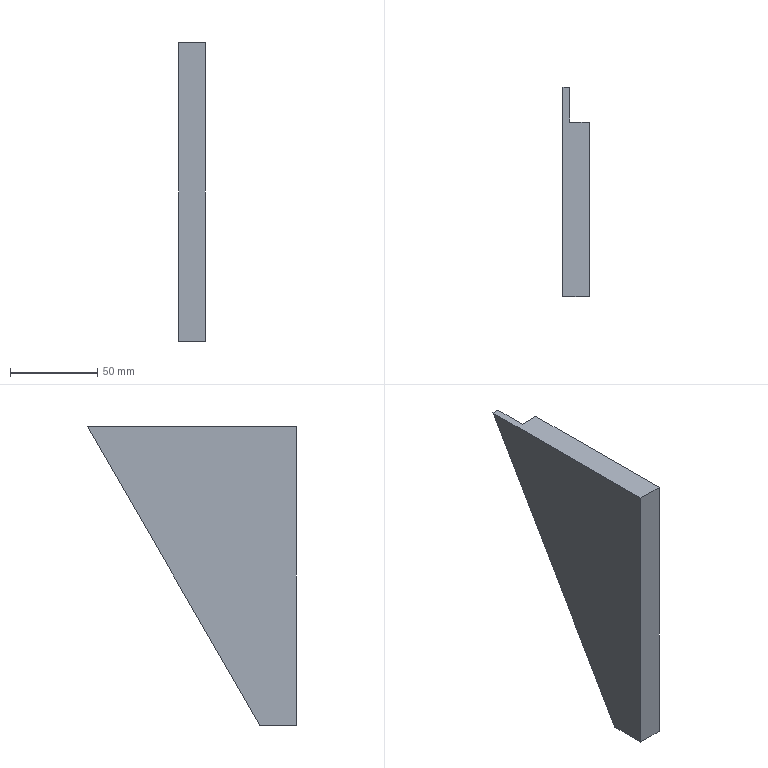Part | STEP file | 02-21 Push plate | 1 solid | 16 faces | box 15 x 120 x 171.5 mm | volume 143256 mm3 | plane 8 | cylinder 4 | cone 4 | commonest cylinder face diameters 4.2 x4
STEP:
#1=CARTESIAN_POINT('',(0.,0.,0.));
#2=DIRECTION('',(0.,0.,1.));
#3=DIRECTION('',(1.,0.,0.));
#4=AXIS2_PLACEMENT_3D('',#1,#2,#3);
#5=CARTESIAN_POINT('',(2.6,22.5,-67.6));
#6=VERTEX_POINT('',#5);
#7=CARTESIAN_POINT('',(15.,22.5,-67.6));
#8=VERTEX_POINT('',#7);
#9=CARTESIAN_POINT('',(2.6,22.5,-67.6));
#10=DIRECTION('',(1.,0.,0.));
#11=VECTOR('',#10,1.);
#12=LINE('',#9,#11);
#13=CARTESIAN_POINT('',(2.6,22.5,-65.5));
#14=DIRECTION('',(1.,0.,0.));
#15=DIRECTION('',(0.,0.,-1.));
#16=AXIS2_PLACEMENT_3D('',#13,#14,#15);
#17=CYLINDRICAL_SURFACE('',#16,2.1);
#18=CARTESIAN_POINT('',(6.283,0.));
#19=DIRECTION('',(0.,1.));
#20=VECTOR('',#19,1.);
#21=LINE('',#18,#20);
#22=(GEOMETRIC_REPRESENTATION_CONTEXT(2)PARAMETRIC_REPRESENTATION_CONTEXT()REPRESENTATION_CONTEXT('',''));
#23=DEFINITIONAL_REPRESENTATION('',(#21),#22);
#24=PCURVE('',#17,#23);
#25=CARTESIAN_POINT('',(2.6,22.5,-65.5));
#26=DIRECTION('',(1.,0.,0.));
#27=DIRECTION('',(0.,0.,-1.));
#28=AXIS2_PLACEMENT_3D('',#25,#26,#27);
#29=CYLINDRICAL_SURFACE('',#28,2.1);
#30=CARTESIAN_POINT('',(0.,0.));
#31=DIRECTION('',(0.,1.));
#32=VECTOR('',#31,1.);
#33=LINE('',#30,#32);
#34=(GEOMETRIC_REPRESENTATION_CONTEXT(2)PARAMETRIC_REPRESENTATION_CONTEXT()REPRESENTATION_CONTEXT('',''));
#35=DEFINITIONAL_REPRESENTATION('',(#33),#34);
#36=PCURVE('',#29,#35);
#37=SURFACE_CURVE('',#12,(#24,#36),.PCURVE_S1.);
#38=EDGE_CURVE('',#6,#8,#37,.T.);
#39=ORIENTED_EDGE('',*,*,#38,.T.);
#40=CARTESIAN_POINT('',(15.,22.5,-63.4));
#41=VERTEX_POINT('',#40);
#42=CARTESIAN_POINT('',(15.,22.5,-65.5));
#43=DIRECTION('',(1.,0.,0.));
#44=DIRECTION('',(0.,0.,-1.));
#45=AXIS2_PLACEMENT_3D('',#42,#43,#44);
#46=CIRCLE('',#45,2.1);
#47=CARTESIAN_POINT('',(0.,12.4));
#48=DIRECTION('',(1.,0.));
#49=VECTOR('',#48,1.);
#50=LINE('',#47,#49);
#51=(GEOMETRIC_REPRESENTATION_CONTEXT(2)PARAMETRIC_REPRESENTATION_CONTEXT()REPRESENTATION_CONTEXT('',''));
#52=DEFINITIONAL_REPRESENTATION('',(#50),#51);
#53=PCURVE('',#17,#52);
#54=CARTESIAN_POINT('',(15.,0.,-171.5));
#55=DIRECTION('',(-1.,0.,0.));
#56=DIRECTION('',(0.,0.,1.));
#57=AXIS2_PLACEMENT_3D('',#54,#55,#56);
#58=PLANE('',#57);
#59=CARTESIAN_POINT('',(103.9,22.5));
#60=CARTESIAN_POINT('',(103.9,26.137));
#61=CARTESIAN_POINT('',(107.05,24.319));
#62=CARTESIAN_POINT('',(110.2,22.5));
#63=CARTESIAN_POINT('',(107.05,20.681));
#64=CARTESIAN_POINT('',(103.9,18.863));
#65=CARTESIAN_POINT('',(103.9,22.5));
#66=(BOUNDED_CURVE()B_SPLINE_CURVE(2,(#59,#60,#61,#62,#63,#64,#65),.UNSPECIFIED.,.T.,.F.)B_SPLINE_CURVE_WITH_KNOTS((1,2,2,2,2,1),(-2.094,0.,2.094,4.189,6.283,8.378),.UNSPECIFIED.)CURVE()GEOMETRIC_REPRESENTATION_ITEM()RATIONAL_B_SPLINE_CURVE((1.,0.5,1.,0.5,1.,0.5,1.))REPRESENTATION_ITEM(''));
#67=(GEOMETRIC_REPRESENTATION_CONTEXT(2)PARAMETRIC_REPRESENTATION_CONTEXT()REPRESENTATION_CONTEXT('',''));
#68=DEFINITIONAL_REPRESENTATION('',(#66),#67);
#69=PCURVE('',#58,#68);
#70=SURFACE_CURVE('',#46,(#53,#69),.PCURVE_S1.);
#71=EDGE_CURVE('',#41,#8,#70,.T.);
#72=ORIENTED_EDGE('',*,*,#71,.F.);
#73=CARTESIAN_POINT('',(2.6,22.5,-63.4));
#74=VERTEX_POINT('',#73);
#75=CARTESIAN_POINT('',(2.6,22.5,-63.4));
#76=DIRECTION('',(1.,0.,0.));
#77=VECTOR('',#76,1.);
#78=LINE('',#75,#77);
#79=CARTESIAN_POINT('',(3.142,0.));
#80=DIRECTION('',(0.,1.));
#81=VECTOR('',#80,1.);
#82=LINE('',#79,#81);
#83=(GEOMETRIC_REPRESENTATION_CONTEXT(2)PARAMETRIC_REPRESENTATION_CONTEXT()REPRESENTATION_CONTEXT('',''));
#84=DEFINITIONAL_REPRESENTATION('',(#82),#83);
#85=PCURVE('',#17,#84);
#86=CARTESIAN_POINT('',(3.142,0.));
#87=DIRECTION('',(0.,1.));
#88=VECTOR('',#87,1.);
#89=LINE('',#86,#88);
#90=(GEOMETRIC_REPRESENTATION_CONTEXT(2)PARAMETRIC_REPRESENTATION_CONTEXT()REPRESENTATION_CONTEXT('',''));
#91=DEFINITIONAL_REPRESENTATION('',(#89),#90);
#92=PCURVE('',#29,#91);
#93=SURFACE_CURVE('',#78,(#85,#92),.PCURVE_S1.);
#94=EDGE_CURVE('',#74,#41,#93,.T.);
#95=ORIENTED_EDGE('',*,*,#94,.F.);
#96=CARTESIAN_POINT('',(2.6,22.5,-65.5));
#97=DIRECTION('',(-1.,0.,0.));
#98=DIRECTION('',(0.,0.,-1.));
#99=AXIS2_PLACEMENT_3D('',#96,#97,#98);
#100=CIRCLE('',#99,2.1);
#101=CARTESIAN_POINT('',(6.283,0.));
#102=DIRECTION('',(-1.,0.));
#103=VECTOR('',#102,1.);
#104=LINE('',#101,#103);
#105=(GEOMETRIC_REPRESENTATION_CONTEXT(2)PARAMETRIC_REPRESENTATION_CONTEXT()REPRESENTATION_CONTEXT('',''));
#106=DEFINITIONAL_REPRESENTATION('',(#104),#105);
#107=PCURVE('',#17,#106);
#108=CARTESIAN_POINT('',(1001.338,22.5,-65.5));
#109=DIRECTION('',(1.,0.,0.));
#110=DIRECTION('',(0.,0.,-1.));
#111=AXIS2_PLACEMENT_3D('',#108,#109,#110);
#112=CONICAL_SURFACE('',#111,1664.279,1.03);
#113=CARTESIAN_POINT('',(6.283,-998.738));
#114=DIRECTION('',(-1.,0.));
#115=VECTOR('',#114,1.);
#116=LINE('',#113,#115);
#117=(GEOMETRIC_REPRESENTATION_CONTEXT(2)PARAMETRIC_REPRESENTATION_CONTEXT()REPRESENTATION_CONTEXT('',''));
#118=DEFINITIONAL_REPRESENTATION('',(#116),#117);
#119=PCURVE('',#112,#118);
#120=SURFACE_CURVE('',#100,(#107,#119),.PCURVE_S1.);
#121=EDGE_CURVE('',#6,#74,#120,.T.);
#122=ORIENTED_EDGE('',*,*,#121,.F.);
#123=EDGE_LOOP('',(#39,#72,#95,#122));
#124=FACE_BOUND('',#123,.F.);
#125=ADVANCED_FACE('',(#124),#17,.F.);
#126=ORIENTED_EDGE('',*,*,#121,.T.);
#127=CARTESIAN_POINT('',(1.338,22.5,-65.5));
#128=VERTEX_POINT('',#127);
#129=CARTESIAN_POINT('',(1.338,22.5,-65.5));
#130=DIRECTION('',(0.515,0.,0.8572));
#131=VECTOR('',#130,1.);
#132=LINE('',#129,#131);
#133=CARTESIAN_POINT('',(3.142,-1000.));
#134=CARTESIAN_POINT('',(3.142,-999.981));
#135=CARTESIAN_POINT('',(3.142,-999.943));
#136=CARTESIAN_POINT('',(3.142,-999.885));
#137=CARTESIAN_POINT('',(3.142,-999.828));
#138=CARTESIAN_POINT('',(3.142,-999.771));
#139=CARTESIAN_POINT('',(3.142,-999.713));
#140=CARTESIAN_POINT('',(3.142,-999.656));
#141=CARTESIAN_POINT('',(3.142,-999.599));
#142=CARTESIAN_POINT('',(3.142,-999.541));
#143=CARTESIAN_POINT('',(3.142,-999.484));
#144=CARTESIAN_POINT('',(3.142,-999.426));
#145=CARTESIAN_POINT('',(3.142,-999.369));
#146=CARTESIAN_POINT('',(3.142,-999.312));
#147=CARTESIAN_POINT('',(3.142,-999.254));
#148=CARTESIAN_POINT('',(3.142,-999.197));
#149=CARTESIAN_POINT('',(3.142,-999.14));
#150=CARTESIAN_POINT('',(3.142,-999.082));
#151=CARTESIAN_POINT('',(3.142,-999.025));
#152=CARTESIAN_POINT('',(3.142,-998.968));
#153=CARTESIAN_POINT('',(3.142,-998.91));
#154=CARTESIAN_POINT('',(3.142,-998.853));
#155=CARTESIAN_POINT('',(3.142,-998.796));
#156=CARTESIAN_POINT('',(3.142,-998.757));
#157=CARTESIAN_POINT('',(3.142,-998.738));
#158=B_SPLINE_CURVE_WITH_KNOTS('',3,(#133,#134,#135,#136,#137,#138,#139,#140,#141,#142,#143,#144,#145,#146,#147,#148,#149,#150,#151,#152,#153,#154,#155,#156,#157),.UNSPECIFIED.,.F.,.F.,(4,1,1,1,1,1,1,1,1,1,1,1,1,1,1,1,1,1,1,1,1,1,4),(0.,0.1114,0.2227,0.3341,0.4454,0.5568,0.6682,0.7795,0.8909,1.002,1.114,1.225,1.336,1.448,1.559,1.67,1.782,1.893,2.004,2.116,2.227,2.339,2.45),.QUASI_UNIFORM_KNOTS.);
#159=(GEOMETRIC_REPRESENTATION_CONTEXT(2)PARAMETRIC_REPRESENTATION_CONTEXT()REPRESENTATION_CONTEXT('',''));
#160=DEFINITIONAL_REPRESENTATION('',(#158),#159);
#161=PCURVE('',#112,#160);
#162=CARTESIAN_POINT('',(1001.338,22.5,-65.5));
#163=DIRECTION('',(1.,0.,0.));
#164=DIRECTION('',(0.,0.,-1.));
#165=AXIS2_PLACEMENT_3D('',#162,#163,#164);
#166=CONICAL_SURFACE('',#165,1664.279,1.03);
#167=CARTESIAN_POINT('',(3.142,-1000.));
#168=CARTESIAN_POINT('',(3.142,-999.981));
#169=CARTESIAN_POINT('',(3.142,-999.943));
#170=CARTESIAN_POINT('',(3.142,-999.885));
#171=CARTESIAN_POINT('',(3.142,-999.828));
#172=CARTESIAN_POINT('',(3.142,-999.771));
#173=CARTESIAN_POINT('',(3.142,-999.713));
#174=CARTESIAN_POINT('',(3.142,-999.656));
#175=CARTESIAN_POINT('',(3.142,-999.599));
#176=CARTESIAN_POINT('',(3.142,-999.541));
#177=CARTESIAN_POINT('',(3.142,-999.484));
#178=CARTESIAN_POINT('',(3.142,-999.426));
#179=CARTESIAN_POINT('',(3.142,-999.369));
#180=CARTESIAN_POINT('',(3.142,-999.312));
#181=CARTESIAN_POINT('',(3.142,-999.254));
#182=CARTESIAN_POINT('',(3.142,-999.197));
#183=CARTESIAN_POINT('',(3.142,-999.14));
#184=CARTESIAN_POINT('',(3.142,-999.082));
#185=CARTESIAN_POINT('',(3.142,-999.025));
#186=CARTESIAN_POINT('',(3.142,-998.968));
#187=CARTESIAN_POINT('',(3.142,-998.91));
#188=CARTESIAN_POINT('',(3.142,-998.853));
#189=CARTESIAN_POINT('',(3.142,-998.796));
#190=CARTESIAN_POINT('',(3.142,-998.757));
#191=CARTESIAN_POINT('',(3.142,-998.738));
#192=B_SPLINE_CURVE_WITH_KNOTS('',3,(#167,#168,#169,#170,#171,#172,#173,#174,#175,#176,#177,#178,#179,#180,#181,#182,#183,#184,#185,#186,#187,#188,#189,#190,#191),.UNSPECIFIED.,.F.,.F.,(4,1,1,1,1,1,1,1,1,1,1,1,1,1,1,1,1,1,1,1,1,1,4),(0.,0.1114,0.2227,0.3341,0.4454,0.5568,0.6682,0.7795,0.8909,1.002,1.114,1.225,1.336,1.448,1.559,1.67,1.782,1.893,2.004,2.116,2.227,2.339,2.45),.QUASI_UNIFORM_KNOTS.);
#193=(GEOMETRIC_REPRESENTATION_CONTEXT(2)PARAMETRIC_REPRESENTATION_CONTEXT()REPRESENTATION_CONTEXT('',''));
#194=DEFINITIONAL_REPRESENTATION('',(#192),#193);
#195=PCURVE('',#166,#194);
#196=SURFACE_CURVE('',#132,(#161,#195),.PCURVE_S1.);
#197=EDGE_CURVE('',#128,#74,#196,.T.);
#198=ORIENTED_EDGE('',*,*,#197,.F.);
#199=CARTESIAN_POINT('',(1.338,22.5,-65.5));
#200=DIRECTION('',(0.515,0.,-0.8572));
#201=VECTOR('',#200,1.);
#202=LINE('',#199,#201);
#203=CARTESIAN_POINT('',(6.283,-1000.));
#204=DIRECTION('',(0.,1.));
#205=VECTOR('',#204,1.);
#206=LINE('',#203,#205);
#207=(GEOMETRIC_REPRESENTATION_CONTEXT(2)PARAMETRIC_REPRESENTATION_CONTEXT()REPRESENTATION_CONTEXT('',''));
#208=DEFINITIONAL_REPRESENTATION('',(#206),#207);
#209=PCURVE('',#112,#208);
#210=CARTESIAN_POINT('',(0.,-1000.));
#211=DIRECTION('',(0.,1.));
#212=VECTOR('',#211,1.);
#213=LINE('',#210,#212);
#214=(GEOMETRIC_REPRESENTATION_CONTEXT(2)PARAMETRIC_REPRESENTATION_CONTEXT()REPRESENTATION_CONTEXT('',''));
#215=DEFINITIONAL_REPRESENTATION('',(#213),#214);
#216=PCURVE('',#166,#215);
#217=SURFACE_CURVE('',#202,(#209,#216),.PCURVE_S1.);
#218=EDGE_CURVE('',#128,#6,#217,.T.);
#219=ORIENTED_EDGE('',*,*,#218,.T.);
#220=EDGE_LOOP('',(#126,#198,#219));
#221=FACE_BOUND('',#220,.F.);
#222=ADVANCED_FACE('',(#221),#112,.F.);
#223=CARTESIAN_POINT('',(2.6,22.5,-97.6));
#224=VERTEX_POINT('',#223);
#225=CARTESIAN_POINT('',(15.,22.5,-97.6));
#226=VERTEX_POINT('',#225);
#227=CARTESIAN_POINT('',(2.6,22.5,-97.6));
#228=DIRECTION('',(1.,0.,0.));
#229=VECTOR('',#228,1.);
#230=LINE('',#227,#229);
#231=CARTESIAN_POINT('',(2.6,22.5,-95.5));
#232=DIRECTION('',(1.,0.,0.));
#233=DIRECTION('',(0.,0.,-1.));
#234=AXIS2_PLACEMENT_3D('',#231,#232,#233);
#235=CYLINDRICAL_SURFACE('',#234,2.1);
#236=CARTESIAN_POINT('',(6.283,0.));
#237=DIRECTION('',(0.,1.));
#238=VECTOR('',#237,1.);
#239=LINE('',#236,#238);
#240=(GEOMETRIC_REPRESENTATION_CONTEXT(2)PARAMETRIC_REPRESENTATION_CONTEXT()REPRESENTATION_CONTEXT('',''));
#241=DEFINITIONAL_REPRESENTATION('',(#239),#240);
#242=PCURVE('',#235,#241);
#243=CARTESIAN_POINT('',(2.6,22.5,-95.5));
#244=DIRECTION('',(1.,0.,0.));
#245=DIRECTION('',(0.,0.,-1.));
#246=AXIS2_PLACEMENT_3D('',#243,#244,#245);
#247=CYLINDRICAL_SURFACE('',#246,2.1);
#248=CARTESIAN_POINT('',(0.,0.));
#249=DIRECTION('',(0.,1.));
#250=VECTOR('',#249,1.);
#251=LINE('',#248,#250);
#252=(GEOMETRIC_REPRESENTATION_CONTEXT(2)PARAMETRIC_REPRESENTATION_CONTEXT()REPRESENTATION_CONTEXT('',''));
#253=DEFINITIONAL_REPRESENTATION('',(#251),#252);
#254=PCURVE('',#247,#253);
#255=SURFACE_CURVE('',#230,(#242,#254),.PCURVE_S1.);
#256=EDGE_CURVE('',#224,#226,#255,.T.);
#257=ORIENTED_EDGE('',*,*,#256,.T.);
#258=CARTESIAN_POINT('',(15.,22.5,-93.4));
#259=VERTEX_POINT('',#258);
#260=CARTESIAN_POINT('',(15.,22.5,-95.5));
#261=DIRECTION('',(1.,0.,0.));
#262=DIRECTION('',(0.,0.,-1.));
#263=AXIS2_PLACEMENT_3D('',#260,#261,#262);
#264=CIRCLE('',#263,2.1);
#265=CARTESIAN_POINT('',(0.,12.4));
#266=DIRECTION('',(1.,0.));
#267=VECTOR('',#266,1.);
#268=LINE('',#265,#267);
#269=(GEOMETRIC_REPRESENTATION_CONTEXT(2)PARAMETRIC_REPRESENTATION_CONTEXT()REPRESENTATION_CONTEXT('',''));
#270=DEFINITIONAL_REPRESENTATION('',(#268),#269);
#271=PCURVE('',#235,#270);
#272=CARTESIAN_POINT('',(73.9,22.5));
#273=CARTESIAN_POINT('',(73.9,26.137));
#274=CARTESIAN_POINT('',(77.05,24.319));
#275=CARTESIAN_POINT('',(80.2,22.5));
#276=CARTESIAN_POINT('',(77.05,20.681));
#277=CARTESIAN_POINT('',(73.9,18.863));
#278=CARTESIAN_POINT('',(73.9,22.5));
#279=(BOUNDED_CURVE()B_SPLINE_CURVE(2,(#272,#273,#274,#275,#276,#277,#278),.UNSPECIFIED.,.T.,.F.)B_SPLINE_CURVE_WITH_KNOTS((1,2,2,2,2,1),(-2.094,0.,2.094,4.189,6.283,8.378),.UNSPECIFIED.)CURVE()GEOMETRIC_REPRESENTATION_ITEM()RATIONAL_B_SPLINE_CURVE((1.,0.5,1.,0.5,1.,0.5,1.))REPRESENTATION_ITEM(''));
#280=(GEOMETRIC_REPRESENTATION_CONTEXT(2)PARAMETRIC_REPRESENTATION_CONTEXT()REPRESENTATION_CONTEXT('',''));
#281=DEFINITIONAL_REPRESENTATION('',(#279),#280);
#282=PCURVE('',#58,#281);
#283=SURFACE_CURVE('',#264,(#271,#282),.PCURVE_S1.);
#284=EDGE_CURVE('',#259,#226,#283,.T.);
#285=ORIENTED_EDGE('',*,*,#284,.F.);
#286=CARTESIAN_POINT('',(2.6,22.5,-93.4));
#287=VERTEX_POINT('',#286);
#288=CARTESIAN_POINT('',(2.6,22.5,-93.4));
#289=DIRECTION('',(1.,0.,0.));
#290=VECTOR('',#289,1.);
#291=LINE('',#288,#290);
#292=CARTESIAN_POINT('',(3.142,0.));
#293=DIRECTION('',(0.,1.));
#294=VECTOR('',#293,1.);
#295=LINE('',#292,#294);
#296=(GEOMETRIC_REPRESENTATION_CONTEXT(2)PARAMETRIC_REPRESENTATION_CONTEXT()REPRESENTATION_CONTEXT('',''));
#297=DEFINITIONAL_REPRESENTATION('',(#295),#296);
#298=PCURVE('',#235,#297);
#299=CARTESIAN_POINT('',(3.142,0.));
#300=DIRECTION('',(0.,1.));
#301=VECTOR('',#300,1.);
#302=LINE('',#299,#301);
#303=(GEOMETRIC_REPRESENTATION_CONTEXT(2)PARAMETRIC_REPRESENTATION_CONTEXT()REPRESENTATION_CONTEXT('',''));
#304=DEFINITIONAL_REPRESENTATION('',(#302),#303);
#305=PCURVE('',#247,#304);
#306=SURFACE_CURVE('',#291,(#298,#305),.PCURVE_S1.);
#307=EDGE_CURVE('',#287,#259,#306,.T.);
#308=ORIENTED_EDGE('',*,*,#307,.F.);
#309=CARTESIAN_POINT('',(2.6,22.5,-95.5));
#310=DIRECTION('',(-1.,0.,0.));
#311=DIRECTION('',(0.,0.,-1.));
#312=AXIS2_PLACEMENT_3D('',#309,#310,#311);
#313=CIRCLE('',#312,2.1);
#314=CARTESIAN_POINT('',(6.283,0.));
#315=DIRECTION('',(-1.,0.));
#316=VECTOR('',#315,1.);
#317=LINE('',#314,#316);
#318=(GEOMETRIC_REPRESENTATION_CONTEXT(2)PARAMETRIC_REPRESENTATION_CONTEXT()REPRESENTATION_CONTEXT('',''));
#319=DEFINITIONAL_REPRESENTATION('',(#317),#318);
#320=PCURVE('',#235,#319);
#321=CARTESIAN_POINT('',(1001.338,22.5,-95.5));
#322=DIRECTION('',(1.,0.,0.));
#323=DIRECTION('',(0.,0.,-1.));
#324=AXIS2_PLACEMENT_3D('',#321,#322,#323);
#325=CONICAL_SURFACE('',#324,1664.279,1.03);
#326=CARTESIAN_POINT('',(6.283,-998.738));
#327=DIRECTION('',(-1.,0.));
#328=VECTOR('',#327,1.);
#329=LINE('',#326,#328);
#330=(GEOMETRIC_REPRESENTATION_CONTEXT(2)PARAMETRIC_REPRESENTATION_CONTEXT()REPRESENTATION_CONTEXT('',''));
#331=DEFINITIONAL_REPRESENTATION('',(#329),#330);
#332=PCURVE('',#325,#331);
#333=SURFACE_CURVE('',#313,(#320,#332),.PCURVE_S1.);
#334=EDGE_CURVE('',#224,#287,#333,.T.);
#335=ORIENTED_EDGE('',*,*,#334,.F.);
#336=EDGE_LOOP('',(#257,#285,#308,#335));
#337=FACE_BOUND('',#336,.F.);
#338=ADVANCED_FACE('',(#337),#235,.F.);
#339=ORIENTED_EDGE('',*,*,#334,.T.);
#340=CARTESIAN_POINT('',(1.338,22.5,-95.5));
#341=VERTEX_POINT('',#340);
#342=CARTESIAN_POINT('',(1.338,22.5,-95.5));
#343=DIRECTION('',(0.515,0.,0.8572));
#344=VECTOR('',#343,1.);
#345=LINE('',#342,#344);
#346=CARTESIAN_POINT('',(3.142,-1000.));
#347=CARTESIAN_POINT('',(3.142,-999.981));
#348=CARTESIAN_POINT('',(3.142,-999.943));
#349=CARTESIAN_POINT('',(3.142,-999.885));
#350=CARTESIAN_POINT('',(3.142,-999.828));
#351=CARTESIAN_POINT('',(3.142,-999.771));
#352=CARTESIAN_POINT('',(3.142,-999.713));
#353=CARTESIAN_POINT('',(3.142,-999.656));
#354=CARTESIAN_POINT('',(3.142,-999.599));
#355=CARTESIAN_POINT('',(3.142,-999.541));
#356=CARTESIAN_POINT('',(3.142,-999.484));
#357=CARTESIAN_POINT('',(3.142,-999.426));
#358=CARTESIAN_POINT('',(3.142,-999.369));
#359=CARTESIAN_POINT('',(3.142,-999.312));
#360=CARTESIAN_POINT('',(3.142,-999.254));
#361=CARTESIAN_POINT('',(3.142,-999.197));
#362=CARTESIAN_POINT('',(3.142,-999.14));
#363=CARTESIAN_POINT('',(3.142,-999.082));
#364=CARTESIAN_POINT('',(3.142,-999.025));
#365=CARTESIAN_POINT('',(3.142,-998.968));
#366=CARTESIAN_POINT('',(3.142,-998.91));
#367=CARTESIAN_POINT('',(3.142,-998.853));
#368=CARTESIAN_POINT('',(3.142,-998.796));
#369=CARTESIAN_POINT('',(3.142,-998.757));
#370=CARTESIAN_POINT('',(3.142,-998.738));
#371=B_SPLINE_CURVE_WITH_KNOTS('',3,(#346,#347,#348,#349,#350,#351,#352,#353,#354,#355,#356,#357,#358,#359,#360,#361,#362,#363,#364,#365,#366,#367,#368,#369,#370),.UNSPECIFIED.,.F.,.F.,(4,1,1,1,1,1,1,1,1,1,1,1,1,1,1,1,1,1,1,1,1,1,4),(0.,0.1114,0.2227,0.3341,0.4454,0.5568,0.6682,0.7795,0.8909,1.002,1.114,1.225,1.336,1.448,1.559,1.67,1.782,1.893,2.004,2.116,2.227,2.339,2.45),.UNSPECIFIED.);
#372=(GEOMETRIC_REPRESENTATION_CONTEXT(2)PARAMETRIC_REPRESENTATION_CONTEXT()REPRESENTATION_CONTEXT('',''));
#373=DEFINITIONAL_REPRESENTATION('',(#371),#372);
#374=PCURVE('',#325,#373);
#375=CARTESIAN_POINT('',(1001.338,22.5,-95.5));
#376=DIRECTION('',(1.,0.,0.));
#377=DIRECTION('',(0.,0.,-1.));
#378=AXIS2_PLACEMENT_3D('',#375,#376,#377);
#379=CONICAL_SURFACE('',#378,1664.279,1.03);
#380=CARTESIAN_POINT('',(3.142,-1000.));
#381=CARTESIAN_POINT('',(3.142,-999.981));
#382=CARTESIAN_POINT('',(3.142,-999.943));
#383=CARTESIAN_POINT('',(3.142,-999.885));
#384=CARTESIAN_POINT('',(3.142,-999.828));
#385=CARTESIAN_POINT('',(3.142,-999.771));
#386=CARTESIAN_POINT('',(3.142,-999.713));
#387=CARTESIAN_POINT('',(3.142,-999.656));
#388=CARTESIAN_POINT('',(3.142,-999.599));
#389=CARTESIAN_POINT('',(3.142,-999.541));
#390=CARTESIAN_POINT('',(3.142,-999.484));
#391=CARTESIAN_POINT('',(3.142,-999.426));
#392=CARTESIAN_POINT('',(3.142,-999.369));
#393=CARTESIAN_POINT('',(3.142,-999.312));
#394=CARTESIAN_POINT('',(3.142,-999.254));
#395=CARTESIAN_POINT('',(3.142,-999.197));
#396=CARTESIAN_POINT('',(3.142,-999.14));
#397=CARTESIAN_POINT('',(3.142,-999.082));
#398=CARTESIAN_POINT('',(3.142,-999.025));
#399=CARTESIAN_POINT('',(3.142,-998.968));
#400=CARTESIAN_POINT('',(3.142,-998.91));
#401=CARTESIAN_POINT('',(3.142,-998.853));
#402=CARTESIAN_POINT('',(3.142,-998.796));
#403=CARTESIAN_POINT('',(3.142,-998.757));
#404=CARTESIAN_POINT('',(3.142,-998.738));
#405=B_SPLINE_CURVE_WITH_KNOTS('',3,(#380,#381,#382,#383,#384,#385,#386,#387,#388,#389,#390,#391,#392,#393,#394,#395,#396,#397,#398,#399,#400,#401,#402,#403,#404),.UNSPECIFIED.,.F.,.F.,(4,1,1,1,1,1,1,1,1,1,1,1,1,1,1,1,1,1,1,1,1,1,4),(0.,0.1114,0.2227,0.3341,0.4454,0.5568,0.6682,0.7795,0.8909,1.002,1.114,1.225,1.336,1.448,1.559,1.67,1.782,1.893,2.004,2.116,2.227,2.339,2.45),.UNSPECIFIED.);
#406=(GEOMETRIC_REPRESENTATION_CONTEXT(2)PARAMETRIC_REPRESENTATION_CONTEXT()REPRESENTATION_CONTEXT('',''));
#407=DEFINITIONAL_REPRESENTATION('',(#405),#406);
#408=PCURVE('',#379,#407);
#409=SURFACE_CURVE('',#345,(#374,#408),.PCURVE_S1.);
#410=EDGE_CURVE('',#341,#287,#409,.T.);
#411=ORIENTED_EDGE('',*,*,#410,.F.);
#412=CARTESIAN_POINT('',(1.338,22.5,-95.5));
#413=DIRECTION('',(0.515,0.,-0.8572));
#414=VECTOR('',#413,1.);
#415=LINE('',#412,#414);
#416=CARTESIAN_POINT('',(6.283,-1000.));
#417=DIRECTION('',(0.,1.));
#418=VECTOR('',#417,1.);
#419=LINE('',#416,#418);
#420=(GEOMETRIC_REPRESENTATION_CONTEXT(2)PARAMETRIC_REPRESENTATION_CONTEXT()REPRESENTATION_CONTEXT('',''));
#421=DEFINITIONAL_REPRESENTATION('',(#419),#420);
#422=PCURVE('',#325,#421);
#423=CARTESIAN_POINT('',(0.,-1000.));
#424=DIRECTION('',(0.,1.));
#425=VECTOR('',#424,1.);
#426=LINE('',#423,#425);
#427=(GEOMETRIC_REPRESENTATION_CONTEXT(2)PARAMETRIC_REPRESENTATION_CONTEXT()REPRESENTATION_CONTEXT('',''));
#428=DEFINITIONAL_REPRESENTATION('',(#426),#427);
#429=PCURVE('',#379,#428);
#430=SURFACE_CURVE('',#415,(#422,#429),.PCURVE_S1.);
#431=EDGE_CURVE('',#341,#224,#430,.T.);
#432=ORIENTED_EDGE('',*,*,#431,.T.);
#433=EDGE_LOOP('',(#339,#411,#432));
#434=FACE_BOUND('',#433,.F.);
#435=ADVANCED_FACE('',(#434),#325,.F.);
#436=CARTESIAN_POINT('',(15.,22.5,-65.5));
#437=DIRECTION('',(1.,0.,0.));
#438=DIRECTION('',(0.,0.,-1.));
#439=AXIS2_PLACEMENT_3D('',#436,#437,#438);
#440=CIRCLE('',#439,2.1);
#441=CARTESIAN_POINT('',(0.,12.4));
#442=DIRECTION('',(1.,0.));
#443=VECTOR('',#442,1.);
#444=LINE('',#441,#443);
#445=(GEOMETRIC_REPRESENTATION_CONTEXT(2)PARAMETRIC_REPRESENTATION_CONTEXT()REPRESENTATION_CONTEXT('',''));
#446=DEFINITIONAL_REPRESENTATION('',(#444),#445);
#447=PCURVE('',#29,#446);
#448=CARTESIAN_POINT('',(103.9,22.5));
#449=CARTESIAN_POINT('',(103.9,26.137));
#450=CARTESIAN_POINT('',(107.05,24.319));
#451=CARTESIAN_POINT('',(110.2,22.5));
#452=CARTESIAN_POINT('',(107.05,20.681));
#453=CARTESIAN_POINT('',(103.9,18.863));
#454=CARTESIAN_POINT('',(103.9,22.5));
#455=(BOUNDED_CURVE()B_SPLINE_CURVE(2,(#448,#449,#450,#451,#452,#453,#454),.UNSPECIFIED.,.T.,.F.)B_SPLINE_CURVE_WITH_KNOTS((1,2,2,2,2,1),(-2.094,0.,2.094,4.189,6.283,8.378),.UNSPECIFIED.)CURVE()GEOMETRIC_REPRESENTATION_ITEM()RATIONAL_B_SPLINE_CURVE((1.,0.5,1.,0.5,1.,0.5,1.))REPRESENTATION_ITEM(''));
#456=(GEOMETRIC_REPRESENTATION_CONTEXT(2)PARAMETRIC_REPRESENTATION_CONTEXT()REPRESENTATION_CONTEXT('',''));
#457=DEFINITIONAL_REPRESENTATION('',(#455),#456);
#458=PCURVE('',#58,#457);
#459=SURFACE_CURVE('',#440,(#447,#458),.PCURVE_S1.);
#460=EDGE_CURVE('',#8,#41,#459,.T.);
#461=ORIENTED_EDGE('',*,*,#460,.F.);
#462=ORIENTED_EDGE('',*,*,#38,.F.);
#463=CARTESIAN_POINT('',(2.6,22.5,-65.5));
#464=DIRECTION('',(-1.,0.,0.));
#465=DIRECTION('',(0.,0.,-1.));
#466=AXIS2_PLACEMENT_3D('',#463,#464,#465);
#467=CIRCLE('',#466,2.1);
#468=CARTESIAN_POINT('',(6.283,0.));
#469=DIRECTION('',(-1.,0.));
#470=VECTOR('',#469,1.);
#471=LINE('',#468,#470);
#472=(GEOMETRIC_REPRESENTATION_CONTEXT(2)PARAMETRIC_REPRESENTATION_CONTEXT()REPRESENTATION_CONTEXT('',''));
#473=DEFINITIONAL_REPRESENTATION('',(#471),#472);
#474=PCURVE('',#29,#473);
#475=CARTESIAN_POINT('',(6.283,-998.738));
#476=DIRECTION('',(-1.,0.));
#477=VECTOR('',#476,1.);
#478=LINE('',#475,#477);
#479=(GEOMETRIC_REPRESENTATION_CONTEXT(2)PARAMETRIC_REPRESENTATION_CONTEXT()REPRESENTATION_CONTEXT('',''));
#480=DEFINITIONAL_REPRESENTATION('',(#478),#479);
#481=PCURVE('',#166,#480);
#482=SURFACE_CURVE('',#467,(#474,#481),.PCURVE_S1.);
#483=EDGE_CURVE('',#74,#6,#482,.T.);
#484=ORIENTED_EDGE('',*,*,#483,.F.);
#485=ORIENTED_EDGE('',*,*,#94,.T.);
#486=EDGE_LOOP('',(#461,#462,#484,#485));
#487=FACE_BOUND('',#486,.F.);
#488=ADVANCED_FACE('',(#487),#29,.F.);
#489=CARTESIAN_POINT('',(15.,22.5,-95.5));
#490=DIRECTION('',(1.,0.,0.));
#491=DIRECTION('',(0.,0.,-1.));
#492=AXIS2_PLACEMENT_3D('',#489,#490,#491);
#493=CIRCLE('',#492,2.1);
#494=CARTESIAN_POINT('',(73.9,22.5));
#495=CARTESIAN_POINT('',(73.9,26.137));
#496=CARTESIAN_POINT('',(77.05,24.319));
#497=CARTESIAN_POINT('',(80.2,22.5));
#498=CARTESIAN_POINT('',(77.05,20.681));
#499=CARTESIAN_POINT('',(73.9,18.863));
#500=CARTESIAN_POINT('',(73.9,22.5));
#501=(BOUNDED_CURVE()B_SPLINE_CURVE(2,(#494,#495,#496,#497,#498,#499,#500),.UNSPECIFIED.,.T.,.F.)B_SPLINE_CURVE_WITH_KNOTS((1,2,2,2,2,1),(-2.094,0.,2.094,4.189,6.283,8.378),.UNSPECIFIED.)CURVE()GEOMETRIC_REPRESENTATION_ITEM()RATIONAL_B_SPLINE_CURVE((1.,0.5,1.,0.5,1.,0.5,1.))REPRESENTATION_ITEM(''));
#502=(GEOMETRIC_REPRESENTATION_CONTEXT(2)PARAMETRIC_REPRESENTATION_CONTEXT()REPRESENTATION_CONTEXT('',''));
#503=DEFINITIONAL_REPRESENTATION('',(#501),#502);
#504=PCURVE('',#58,#503);
#505=CARTESIAN_POINT('',(0.,12.4));
#506=DIRECTION('',(1.,0.));
#507=VECTOR('',#506,1.);
#508=LINE('',#505,#507);
#509=(GEOMETRIC_REPRESENTATION_CONTEXT(2)PARAMETRIC_REPRESENTATION_CONTEXT()REPRESENTATION_CONTEXT('',''));
#510=DEFINITIONAL_REPRESENTATION('',(#508),#509);
#511=PCURVE('',#247,#510);
#512=SURFACE_CURVE('',#493,(#504,#511),.PCURVE_S1.);
#513=EDGE_CURVE('',#226,#259,#512,.T.);
#514=ORIENTED_EDGE('',*,*,#513,.F.);
#515=ORIENTED_EDGE('',*,*,#284,.F.);
#516=EDGE_LOOP('',(#514,#515));
#517=FACE_BOUND('',#516,.T.);
#518=ORIENTED_EDGE('',*,*,#460,.F.);
#519=ORIENTED_EDGE('',*,*,#71,.F.);
#520=EDGE_LOOP('',(#518,#519));
#521=FACE_BOUND('',#520,.T.);
#522=CARTESIAN_POINT('',(15.,100.,0.));
#523=VERTEX_POINT('',#522);
#524=CARTESIAN_POINT('',(15.,0.9844,-171.5));
#525=VERTEX_POINT('',#524);
#526=CARTESIAN_POINT('',(15.,100.,0.));
#527=DIRECTION('',(0.,-0.5,-0.866));
#528=VECTOR('',#527,1.);
#529=LINE('',#526,#528);
#530=CARTESIAN_POINT('',(171.5,100.));
#531=DIRECTION('',(-0.866,-0.5));
#532=VECTOR('',#531,1.);
#533=LINE('',#530,#532);
#534=(GEOMETRIC_REPRESENTATION_CONTEXT(2)PARAMETRIC_REPRESENTATION_CONTEXT()REPRESENTATION_CONTEXT('',''));
#535=DEFINITIONAL_REPRESENTATION('',(#533),#534);
#536=PCURVE('',#58,#535);
#537=CARTESIAN_POINT('',(4.,100.,0.));
#538=DIRECTION('',(0.,-0.866,0.5));
#539=DIRECTION('',(0.,-0.5,-0.866));
#540=AXIS2_PLACEMENT_3D('',#537,#538,#539);
#541=PLANE('',#540);
#542=CARTESIAN_POINT('',(0.,11.));
#543=DIRECTION('',(1.,0.));
#544=VECTOR('',#543,1.);
#545=LINE('',#542,#544);
#546=(GEOMETRIC_REPRESENTATION_CONTEXT(2)PARAMETRIC_REPRESENTATION_CONTEXT()REPRESENTATION_CONTEXT('',''));
#547=DEFINITIONAL_REPRESENTATION('',(#545),#546);
#548=PCURVE('',#541,#547);
#549=SURFACE_CURVE('',#529,(#536,#548),.PCURVE_S1.);
#550=EDGE_CURVE('',#523,#525,#549,.T.);
#551=ORIENTED_EDGE('',*,*,#550,.F.);
#552=CARTESIAN_POINT('',(15.,0.,0.));
#553=VERTEX_POINT('',#552);
#554=CARTESIAN_POINT('',(15.,50.3,0.));
#555=DIRECTION('',(0.,1.,0.));
#556=VECTOR('',#555,1.);
#557=LINE('',#554,#556);
#558=CARTESIAN_POINT('',(171.5,50.3));
#559=DIRECTION('',(0.,1.));
#560=VECTOR('',#559,1.);
#561=LINE('',#558,#560);
#562=(GEOMETRIC_REPRESENTATION_CONTEXT(2)PARAMETRIC_REPRESENTATION_CONTEXT()REPRESENTATION_CONTEXT('',''));
#563=DEFINITIONAL_REPRESENTATION('',(#561),#562);
#564=PCURVE('',#58,#563);
#565=CARTESIAN_POINT('',(15.,0.,0.));
#566=DIRECTION('',(0.,0.,-1.));
#567=DIRECTION('',(-1.,0.,0.));
#568=AXIS2_PLACEMENT_3D('',#565,#566,#567);
#569=PLANE('',#568);
#570=CARTESIAN_POINT('',(0.,50.3));
#571=DIRECTION('',(0.,1.));
#572=VECTOR('',#571,1.);
#573=LINE('',#570,#572);
#574=(GEOMETRIC_REPRESENTATION_CONTEXT(2)PARAMETRIC_REPRESENTATION_CONTEXT()REPRESENTATION_CONTEXT('',''));
#575=DEFINITIONAL_REPRESENTATION('',(#573),#574);
#576=PCURVE('',#569,#575);
#577=SURFACE_CURVE('',#557,(#564,#576),.PCURVE_S1.);
#578=EDGE_CURVE('',#553,#523,#577,.T.);
#579=ORIENTED_EDGE('',*,*,#578,.F.);
#580=CARTESIAN_POINT('',(15.,0.,-171.5));
#581=VERTEX_POINT('',#580);
#582=CARTESIAN_POINT('',(15.,0.,-85.75));
#583=DIRECTION('',(0.,0.,1.));
#584=VECTOR('',#583,1.);
#585=LINE('',#582,#584);
#586=CARTESIAN_POINT('',(85.75,0.));
#587=DIRECTION('',(1.,0.));
#588=VECTOR('',#587,1.);
#589=LINE('',#586,#588);
#590=(GEOMETRIC_REPRESENTATION_CONTEXT(2)PARAMETRIC_REPRESENTATION_CONTEXT()REPRESENTATION_CONTEXT('',''));
#591=DEFINITIONAL_REPRESENTATION('',(#589),#590);
#592=PCURVE('',#58,#591);
#593=CARTESIAN_POINT('',(0.,0.,-171.5));
#594=DIRECTION('',(0.,1.,0.));
#595=DIRECTION('',(0.,0.,1.));
#596=AXIS2_PLACEMENT_3D('',#593,#594,#595);
#597=PLANE('',#596);
#598=CARTESIAN_POINT('',(85.75,15.));
#599=DIRECTION('',(1.,0.));
#600=VECTOR('',#599,1.);
#601=LINE('',#598,#600);
#602=(GEOMETRIC_REPRESENTATION_CONTEXT(2)PARAMETRIC_REPRESENTATION_CONTEXT()REPRESENTATION_CONTEXT('',''));
#603=DEFINITIONAL_REPRESENTATION('',(#601),#602);
#604=PCURVE('',#597,#603);
#605=SURFACE_CURVE('',#585,(#592,#604),.PCURVE_S1.);
#606=EDGE_CURVE('',#581,#553,#605,.T.);
#607=ORIENTED_EDGE('',*,*,#606,.F.);
#608=CARTESIAN_POINT('',(15.,10.492,-171.5));
#609=DIRECTION('',(0.,1.,0.));
#610=VECTOR('',#609,1.);
#611=LINE('',#608,#610);
#612=CARTESIAN_POINT('',(0.,10.492));
#613=DIRECTION('',(0.,1.));
#614=VECTOR('',#613,1.);
#615=LINE('',#612,#614);
#616=(GEOMETRIC_REPRESENTATION_CONTEXT(2)PARAMETRIC_REPRESENTATION_CONTEXT()REPRESENTATION_CONTEXT('',''));
#617=DEFINITIONAL_REPRESENTATION('',(#615),#616);
#618=PCURVE('',#58,#617);
#619=CARTESIAN_POINT('',(0.,20.984,-171.5));
#620=DIRECTION('',(0.,0.,1.));
#621=DIRECTION('',(0.,-1.,0.));
#622=AXIS2_PLACEMENT_3D('',#619,#620,#621);
#623=PLANE('',#622);
#624=CARTESIAN_POINT('',(10.492,15.));
#625=DIRECTION('',(-1.,0.));
#626=VECTOR('',#625,1.);
#627=LINE('',#624,#626);
#628=(GEOMETRIC_REPRESENTATION_CONTEXT(2)PARAMETRIC_REPRESENTATION_CONTEXT()REPRESENTATION_CONTEXT('',''));
#629=DEFINITIONAL_REPRESENTATION('',(#627),#628);
#630=PCURVE('',#623,#629);
#631=SURFACE_CURVE('',#611,(#618,#630),.PCURVE_S1.);
#632=EDGE_CURVE('',#581,#525,#631,.T.);
#633=ORIENTED_EDGE('',*,*,#632,.T.);
#634=EDGE_LOOP('',(#551,#579,#607,#633));
#635=FACE_BOUND('',#634,.T.);
#636=ADVANCED_FACE('',(#517,#521,#635),#58,.F.);
#637=ORIENTED_EDGE('',*,*,#483,.T.);
#638=ORIENTED_EDGE('',*,*,#218,.F.);
#639=ORIENTED_EDGE('',*,*,#197,.T.);
#640=EDGE_LOOP('',(#637,#638,#639));
#641=FACE_BOUND('',#640,.F.);
#642=ADVANCED_FACE('',(#641),#166,.F.);
#643=ORIENTED_EDGE('',*,*,#513,.F.);
#644=ORIENTED_EDGE('',*,*,#256,.F.);
#645=CARTESIAN_POINT('',(2.6,22.5,-95.5));
#646=DIRECTION('',(-1.,0.,0.));
#647=DIRECTION('',(0.,0.,-1.));
#648=AXIS2_PLACEMENT_3D('',#645,#646,#647);
#649=CIRCLE('',#648,2.1);
#650=CARTESIAN_POINT('',(6.283,0.));
#651=DIRECTION('',(-1.,0.));
#652=VECTOR('',#651,1.);
#653=LINE('',#650,#652);
#654=(GEOMETRIC_REPRESENTATION_CONTEXT(2)PARAMETRIC_REPRESENTATION_CONTEXT()REPRESENTATION_CONTEXT('',''));
#655=DEFINITIONAL_REPRESENTATION('',(#653),#654);
#656=PCURVE('',#247,#655);
#657=CARTESIAN_POINT('',(6.283,-998.738));
#658=DIRECTION('',(-1.,0.));
#659=VECTOR('',#658,1.);
#660=LINE('',#657,#659);
#661=(GEOMETRIC_REPRESENTATION_CONTEXT(2)PARAMETRIC_REPRESENTATION_CONTEXT()REPRESENTATION_CONTEXT('',''));
#662=DEFINITIONAL_REPRESENTATION('',(#660),#661);
#663=PCURVE('',#379,#662);
#664=SURFACE_CURVE('',#649,(#656,#663),.PCURVE_S1.);
#665=EDGE_CURVE('',#287,#224,#664,.T.);
#666=ORIENTED_EDGE('',*,*,#665,.F.);
#667=ORIENTED_EDGE('',*,*,#307,.T.);
#668=EDGE_LOOP('',(#643,#644,#666,#667));
#669=FACE_BOUND('',#668,.F.);
#670=ADVANCED_FACE('',(#669),#247,.F.);
#671=CARTESIAN_POINT('',(4.,0.9844,-171.5));
#672=VERTEX_POINT('',#671);
#673=CARTESIAN_POINT('',(9.5,0.9844,-171.5));
#674=DIRECTION('',(1.,0.,0.));
#675=VECTOR('',#674,1.);
#676=LINE('',#673,#675);
#677=CARTESIAN_POINT('',(198.031,5.5));
#678=DIRECTION('',(0.,1.));
#679=VECTOR('',#678,1.);
#680=LINE('',#677,#679);
#681=(GEOMETRIC_REPRESENTATION_CONTEXT(2)PARAMETRIC_REPRESENTATION_CONTEXT()REPRESENTATION_CONTEXT('',''));
#682=DEFINITIONAL_REPRESENTATION('',(#680),#681);
#683=PCURVE('',#541,#682);
#684=CARTESIAN_POINT('',(20.,9.5));
#685=DIRECTION('',(0.,1.));
#686=VECTOR('',#685,1.);
#687=LINE('',#684,#686);
#688=(GEOMETRIC_REPRESENTATION_CONTEXT(2)PARAMETRIC_REPRESENTATION_CONTEXT()REPRESENTATION_CONTEXT('',''));
#689=DEFINITIONAL_REPRESENTATION('',(#687),#688);
#690=PCURVE('',#623,#689);
#691=SURFACE_CURVE('',#676,(#683,#690),.PCURVE_S1.);
#692=EDGE_CURVE('',#672,#525,#691,.T.);
#693=ORIENTED_EDGE('',*,*,#692,.F.);
#694=CARTESIAN_POINT('',(4.,100.,0.));
#695=VERTEX_POINT('',#694);
#696=CARTESIAN_POINT('',(4.,50.492,-85.75));
#697=DIRECTION('',(0.,-0.5,-0.866));
#698=VECTOR('',#697,1.);
#699=LINE('',#696,#698);
#700=CARTESIAN_POINT('',(99.016,0.));
#701=DIRECTION('',(1.,0.));
#702=VECTOR('',#701,1.);
#703=LINE('',#700,#702);
#704=(GEOMETRIC_REPRESENTATION_CONTEXT(2)PARAMETRIC_REPRESENTATION_CONTEXT()REPRESENTATION_CONTEXT('',''));
#705=DEFINITIONAL_REPRESENTATION('',(#703),#704);
#706=PCURVE('',#541,#705);
#707=CARTESIAN_POINT('',(4.,0.2703,0.));
#708=DIRECTION('',(1.,0.,0.));
#709=DIRECTION('',(0.,0.,-1.));
#710=AXIS2_PLACEMENT_3D('',#707,#708,#709);
#711=PLANE('',#710);
#712=CARTESIAN_POINT('',(85.75,50.222));
#713=DIRECTION('',(0.866,-0.5));
#714=VECTOR('',#713,1.);
#715=LINE('',#712,#714);
#716=(GEOMETRIC_REPRESENTATION_CONTEXT(2)PARAMETRIC_REPRESENTATION_CONTEXT()REPRESENTATION_CONTEXT('',''));
#717=DEFINITIONAL_REPRESENTATION('',(#715),#716);
#718=PCURVE('',#711,#717);
#719=SURFACE_CURVE('',#699,(#706,#718),.PCURVE_S1.);
#720=EDGE_CURVE('',#695,#672,#719,.T.);
#721=ORIENTED_EDGE('',*,*,#720,.F.);
#722=CARTESIAN_POINT('',(9.5,100.,0.));
#723=DIRECTION('',(-1.,0.,0.));
#724=VECTOR('',#723,1.);
#725=LINE('',#722,#724);
#726=CARTESIAN_POINT('',(0.,5.5));
#727=DIRECTION('',(0.,-1.));
#728=VECTOR('',#727,1.);
#729=LINE('',#726,#728);
#730=(GEOMETRIC_REPRESENTATION_CONTEXT(2)PARAMETRIC_REPRESENTATION_CONTEXT()REPRESENTATION_CONTEXT('',''));
#731=DEFINITIONAL_REPRESENTATION('',(#729),#730);
#732=PCURVE('',#541,#731);
#733=CARTESIAN_POINT('',(5.5,100.));
#734=DIRECTION('',(1.,0.));
#735=VECTOR('',#734,1.);
#736=LINE('',#733,#735);
#737=(GEOMETRIC_REPRESENTATION_CONTEXT(2)PARAMETRIC_REPRESENTATION_CONTEXT()REPRESENTATION_CONTEXT('',''));
#738=DEFINITIONAL_REPRESENTATION('',(#736),#737);
#739=PCURVE('',#569,#738);
#740=SURFACE_CURVE('',#725,(#732,#739),.PCURVE_S1.);
#741=EDGE_CURVE('',#523,#695,#740,.T.);
#742=ORIENTED_EDGE('',*,*,#741,.F.);
#743=ORIENTED_EDGE('',*,*,#550,.T.);
#744=EDGE_LOOP('',(#693,#721,#742,#743));
#745=FACE_BOUND('',#744,.T.);
#746=ADVANCED_FACE('',(#745),#541,.F.);
#747=ORIENTED_EDGE('',*,*,#741,.T.);
#748=CARTESIAN_POINT('',(4.,120.,0.));
#749=VERTEX_POINT('',#748);
#750=CARTESIAN_POINT('',(4.,60.,0.));
#751=DIRECTION('',(0.,-1.,0.));
#752=VECTOR('',#751,1.);
#753=LINE('',#750,#752);
#754=CARTESIAN_POINT('',(11.,60.));
#755=DIRECTION('',(0.,-1.));
#756=VECTOR('',#755,1.);
#757=LINE('',#754,#756);
#758=(GEOMETRIC_REPRESENTATION_CONTEXT(2)PARAMETRIC_REPRESENTATION_CONTEXT()REPRESENTATION_CONTEXT('',''));
#759=DEFINITIONAL_REPRESENTATION('',(#757),#758);
#760=PCURVE('',#569,#759);
#761=CARTESIAN_POINT('',(0.,59.73));
#762=DIRECTION('',(0.,-1.));
#763=VECTOR('',#762,1.);
#764=LINE('',#761,#763);
#765=(GEOMETRIC_REPRESENTATION_CONTEXT(2)PARAMETRIC_REPRESENTATION_CONTEXT()REPRESENTATION_CONTEXT('',''));
#766=DEFINITIONAL_REPRESENTATION('',(#764),#765);
#767=PCURVE('',#711,#766);
#768=SURFACE_CURVE('',#753,(#760,#767),.PCURVE_S1.);
#769=EDGE_CURVE('',#749,#695,#768,.T.);
#770=ORIENTED_EDGE('',*,*,#769,.F.);
#771=CARTESIAN_POINT('',(0.,120.,0.));
#772=VERTEX_POINT('',#771);
#773=CARTESIAN_POINT('',(7.5,120.,0.));
#774=DIRECTION('',(1.,0.,0.));
#775=VECTOR('',#774,1.);
#776=LINE('',#773,#775);
#777=CARTESIAN_POINT('',(7.5,120.));
#778=DIRECTION('',(-1.,0.));
#779=VECTOR('',#778,1.);
#780=LINE('',#777,#779);
#781=(GEOMETRIC_REPRESENTATION_CONTEXT(2)PARAMETRIC_REPRESENTATION_CONTEXT()REPRESENTATION_CONTEXT('',''));
#782=DEFINITIONAL_REPRESENTATION('',(#780),#781);
#783=PCURVE('',#569,#782);
#784=CARTESIAN_POINT('',(0.,120.,0.));
#785=DIRECTION('',(0.,-0.866,0.5));
#786=DIRECTION('',(0.,-0.5,-0.866));
#787=AXIS2_PLACEMENT_3D('',#784,#785,#786);
#788=PLANE('',#787);
#789=CARTESIAN_POINT('',(0.,7.5));
#790=DIRECTION('',(0.,1.));
#791=VECTOR('',#790,1.);
#792=LINE('',#789,#791);
#793=(GEOMETRIC_REPRESENTATION_CONTEXT(2)PARAMETRIC_REPRESENTATION_CONTEXT()REPRESENTATION_CONTEXT('',''));
#794=DEFINITIONAL_REPRESENTATION('',(#792),#793);
#795=PCURVE('',#788,#794);
#796=SURFACE_CURVE('',#776,(#783,#795),.PCURVE_S1.);
#797=EDGE_CURVE('',#772,#749,#796,.T.);
#798=ORIENTED_EDGE('',*,*,#797,.F.);
#799=CARTESIAN_POINT('',(0.,0.,0.));
#800=VERTEX_POINT('',#799);
#801=CARTESIAN_POINT('',(0.,60.,0.));
#802=DIRECTION('',(0.,1.,0.));
#803=VECTOR('',#802,1.);
#804=LINE('',#801,#803);
#805=CARTESIAN_POINT('',(15.,60.));
#806=DIRECTION('',(0.,1.));
#807=VECTOR('',#806,1.);
#808=LINE('',#805,#807);
#809=(GEOMETRIC_REPRESENTATION_CONTEXT(2)PARAMETRIC_REPRESENTATION_CONTEXT()REPRESENTATION_CONTEXT('',''));
#810=DEFINITIONAL_REPRESENTATION('',(#808),#809);
#811=PCURVE('',#569,#810);
#812=CARTESIAN_POINT('',(0.,0.,-171.5));
#813=DIRECTION('',(-1.,0.,0.));
#814=DIRECTION('',(0.,0.,1.));
#815=AXIS2_PLACEMENT_3D('',#812,#813,#814);
#816=PLANE('',#815);
#817=CARTESIAN_POINT('',(171.5,60.));
#818=DIRECTION('',(0.,1.));
#819=VECTOR('',#818,1.);
#820=LINE('',#817,#819);
#821=(GEOMETRIC_REPRESENTATION_CONTEXT(2)PARAMETRIC_REPRESENTATION_CONTEXT()REPRESENTATION_CONTEXT('',''));
#822=DEFINITIONAL_REPRESENTATION('',(#820),#821);
#823=PCURVE('',#816,#822);
#824=SURFACE_CURVE('',#804,(#811,#823),.PCURVE_S1.);
#825=EDGE_CURVE('',#800,#772,#824,.T.);
#826=ORIENTED_EDGE('',*,*,#825,.F.);
#827=CARTESIAN_POINT('',(7.5,0.,0.));
#828=DIRECTION('',(-1.,0.,0.));
#829=VECTOR('',#828,1.);
#830=LINE('',#827,#829);
#831=CARTESIAN_POINT('',(7.5,0.));
#832=DIRECTION('',(1.,0.));
#833=VECTOR('',#832,1.);
#834=LINE('',#831,#833);
#835=(GEOMETRIC_REPRESENTATION_CONTEXT(2)PARAMETRIC_REPRESENTATION_CONTEXT()REPRESENTATION_CONTEXT('',''));
#836=DEFINITIONAL_REPRESENTATION('',(#834),#835);
#837=PCURVE('',#569,#836);
#838=CARTESIAN_POINT('',(171.5,7.5));
#839=DIRECTION('',(0.,-1.));
#840=VECTOR('',#839,1.);
#841=LINE('',#838,#840);
#842=(GEOMETRIC_REPRESENTATION_CONTEXT(2)PARAMETRIC_REPRESENTATION_CONTEXT()REPRESENTATION_CONTEXT('',''));
#843=DEFINITIONAL_REPRESENTATION('',(#841),#842);
#844=PCURVE('',#597,#843);
#845=SURFACE_CURVE('',#830,(#837,#844),.PCURVE_S1.);
#846=EDGE_CURVE('',#553,#800,#845,.T.);
#847=ORIENTED_EDGE('',*,*,#846,.F.);
#848=ORIENTED_EDGE('',*,*,#578,.T.);
#849=EDGE_LOOP('',(#747,#770,#798,#826,#847,#848));
#850=FACE_BOUND('',#849,.T.);
#851=ADVANCED_FACE('',(#850),#569,.F.);
#852=CARTESIAN_POINT('',(0.,0.,-171.5));
#853=VERTEX_POINT('',#852);
#854=CARTESIAN_POINT('',(7.5,0.,-171.5));
#855=DIRECTION('',(-1.,0.,0.));
#856=VECTOR('',#855,1.);
#857=LINE('',#854,#856);
#858=CARTESIAN_POINT('',(0.,7.5));
#859=DIRECTION('',(0.,-1.));
#860=VECTOR('',#859,1.);
#861=LINE('',#858,#860);
#862=(GEOMETRIC_REPRESENTATION_CONTEXT(2)PARAMETRIC_REPRESENTATION_CONTEXT()REPRESENTATION_CONTEXT('',''));
#863=DEFINITIONAL_REPRESENTATION('',(#861),#862);
#864=PCURVE('',#597,#863);
#865=CARTESIAN_POINT('',(20.984,7.5));
#866=DIRECTION('',(0.,-1.));
#867=VECTOR('',#866,1.);
#868=LINE('',#865,#867);
#869=(GEOMETRIC_REPRESENTATION_CONTEXT(2)PARAMETRIC_REPRESENTATION_CONTEXT()REPRESENTATION_CONTEXT('',''));
#870=DEFINITIONAL_REPRESENTATION('',(#868),#869);
#871=PCURVE('',#623,#870);
#872=SURFACE_CURVE('',#857,(#864,#871),.PCURVE_S1.);
#873=EDGE_CURVE('',#581,#853,#872,.T.);
#874=ORIENTED_EDGE('',*,*,#873,.F.);
#875=ORIENTED_EDGE('',*,*,#606,.T.);
#876=ORIENTED_EDGE('',*,*,#846,.T.);
#877=CARTESIAN_POINT('',(0.,0.,-85.75));
#878=DIRECTION('',(0.,0.,1.));
#879=VECTOR('',#878,1.);
#880=LINE('',#877,#879);
#881=CARTESIAN_POINT('',(85.75,0.));
#882=DIRECTION('',(1.,0.));
#883=VECTOR('',#882,1.);
#884=LINE('',#881,#883);
#885=(GEOMETRIC_REPRESENTATION_CONTEXT(2)PARAMETRIC_REPRESENTATION_CONTEXT()REPRESENTATION_CONTEXT('',''));
#886=DEFINITIONAL_REPRESENTATION('',(#884),#885);
#887=PCURVE('',#597,#886);
#888=CARTESIAN_POINT('',(85.75,0.));
#889=DIRECTION('',(1.,0.));
#890=VECTOR('',#889,1.);
#891=LINE('',#888,#890);
#892=(GEOMETRIC_REPRESENTATION_CONTEXT(2)PARAMETRIC_REPRESENTATION_CONTEXT()REPRESENTATION_CONTEXT('',''));
#893=DEFINITIONAL_REPRESENTATION('',(#891),#892);
#894=PCURVE('',#816,#893);
#895=SURFACE_CURVE('',#880,(#887,#894),.PCURVE_S1.);
#896=EDGE_CURVE('',#853,#800,#895,.T.);
#897=ORIENTED_EDGE('',*,*,#896,.F.);
#898=EDGE_LOOP('',(#874,#875,#876,#897));
#899=FACE_BOUND('',#898,.T.);
#900=ADVANCED_FACE('',(#899),#597,.F.);
#901=ORIENTED_EDGE('',*,*,#665,.T.);
#902=ORIENTED_EDGE('',*,*,#431,.F.);
#903=ORIENTED_EDGE('',*,*,#410,.T.);
#904=EDGE_LOOP('',(#901,#902,#903));
#905=FACE_BOUND('',#904,.F.);
#906=ADVANCED_FACE('',(#905),#379,.F.);
#907=ORIENTED_EDGE('',*,*,#692,.T.);
#908=ORIENTED_EDGE('',*,*,#632,.F.);
#909=ORIENTED_EDGE('',*,*,#873,.T.);
#910=CARTESIAN_POINT('',(0.,20.984,-171.5));
#911=VERTEX_POINT('',#910);
#912=CARTESIAN_POINT('',(0.,10.492,-171.5));
#913=DIRECTION('',(0.,-1.,0.));
#914=VECTOR('',#913,1.);
#915=LINE('',#912,#914);
#916=CARTESIAN_POINT('',(10.492,0.));
#917=DIRECTION('',(1.,0.));
#918=VECTOR('',#917,1.);
#919=LINE('',#916,#918);
#920=(GEOMETRIC_REPRESENTATION_CONTEXT(2)PARAMETRIC_REPRESENTATION_CONTEXT()REPRESENTATION_CONTEXT('',''));
#921=DEFINITIONAL_REPRESENTATION('',(#919),#920);
#922=PCURVE('',#623,#921);
#923=CARTESIAN_POINT('',(0.,10.492));
#924=DIRECTION('',(0.,-1.));
#925=VECTOR('',#924,1.);
#926=LINE('',#923,#925);
#927=(GEOMETRIC_REPRESENTATION_CONTEXT(2)PARAMETRIC_REPRESENTATION_CONTEXT()REPRESENTATION_CONTEXT('',''));
#928=DEFINITIONAL_REPRESENTATION('',(#926),#927);
#929=PCURVE('',#816,#928);
#930=SURFACE_CURVE('',#915,(#922,#929),.PCURVE_S1.);
#931=EDGE_CURVE('',#911,#853,#930,.T.);
#932=ORIENTED_EDGE('',*,*,#931,.F.);
#933=CARTESIAN_POINT('',(4.,20.984,-171.5));
#934=VERTEX_POINT('',#933);
#935=CARTESIAN_POINT('',(7.5,20.984,-171.5));
#936=DIRECTION('',(-1.,0.,0.));
#937=VECTOR('',#936,1.);
#938=LINE('',#935,#937);
#939=CARTESIAN_POINT('',(0.,7.5));
#940=DIRECTION('',(0.,-1.));
#941=VECTOR('',#940,1.);
#942=LINE('',#939,#941);
#943=(GEOMETRIC_REPRESENTATION_CONTEXT(2)PARAMETRIC_REPRESENTATION_CONTEXT()REPRESENTATION_CONTEXT('',''));
#944=DEFINITIONAL_REPRESENTATION('',(#942),#943);
#945=PCURVE('',#623,#944);
#946=CARTESIAN_POINT('',(198.031,7.5));
#947=DIRECTION('',(0.,-1.));
#948=VECTOR('',#947,1.);
#949=LINE('',#946,#948);
#950=(GEOMETRIC_REPRESENTATION_CONTEXT(2)PARAMETRIC_REPRESENTATION_CONTEXT()REPRESENTATION_CONTEXT('',''));
#951=DEFINITIONAL_REPRESENTATION('',(#949),#950);
#952=PCURVE('',#788,#951);
#953=SURFACE_CURVE('',#938,(#945,#952),.PCURVE_S1.);
#954=EDGE_CURVE('',#934,#911,#953,.T.);
#955=ORIENTED_EDGE('',*,*,#954,.F.);
#956=CARTESIAN_POINT('',(4.,10.492,-171.5));
#957=DIRECTION('',(0.,1.,0.));
#958=VECTOR('',#957,1.);
#959=LINE('',#956,#958);
#960=CARTESIAN_POINT('',(10.492,4.));
#961=DIRECTION('',(-1.,0.));
#962=VECTOR('',#961,1.);
#963=LINE('',#960,#962);
#964=(GEOMETRIC_REPRESENTATION_CONTEXT(2)PARAMETRIC_REPRESENTATION_CONTEXT()REPRESENTATION_CONTEXT('',''));
#965=DEFINITIONAL_REPRESENTATION('',(#963),#964);
#966=PCURVE('',#623,#965);
#967=CARTESIAN_POINT('',(171.5,10.222));
#968=DIRECTION('',(0.,1.));
#969=VECTOR('',#968,1.);
#970=LINE('',#967,#969);
#971=(GEOMETRIC_REPRESENTATION_CONTEXT(2)PARAMETRIC_REPRESENTATION_CONTEXT()REPRESENTATION_CONTEXT('',''));
#972=DEFINITIONAL_REPRESENTATION('',(#970),#971);
#973=PCURVE('',#711,#972);
#974=SURFACE_CURVE('',#959,(#966,#973),.PCURVE_S1.);
#975=EDGE_CURVE('',#672,#934,#974,.T.);
#976=ORIENTED_EDGE('',*,*,#975,.F.);
#977=EDGE_LOOP('',(#907,#908,#909,#932,#955,#976));
#978=FACE_BOUND('',#977,.T.);
#979=ADVANCED_FACE('',(#978),#623,.F.);
#980=ORIENTED_EDGE('',*,*,#720,.T.);
#981=ORIENTED_EDGE('',*,*,#975,.T.);
#982=CARTESIAN_POINT('',(4.,20.984,-171.5));
#983=DIRECTION('',(0.,0.5,0.866));
#984=VECTOR('',#983,1.);
#985=LINE('',#982,#984);
#986=CARTESIAN_POINT('',(171.5,20.714));
#987=DIRECTION('',(-0.866,0.5));
#988=VECTOR('',#987,1.);
#989=LINE('',#986,#988);
#990=(GEOMETRIC_REPRESENTATION_CONTEXT(2)PARAMETRIC_REPRESENTATION_CONTEXT()REPRESENTATION_CONTEXT('',''));
#991=DEFINITIONAL_REPRESENTATION('',(#989),#990);
#992=PCURVE('',#711,#991);
#993=CARTESIAN_POINT('',(198.031,4.));
#994=DIRECTION('',(-1.,0.));
#995=VECTOR('',#994,1.);
#996=LINE('',#993,#995);
#997=(GEOMETRIC_REPRESENTATION_CONTEXT(2)PARAMETRIC_REPRESENTATION_CONTEXT()REPRESENTATION_CONTEXT('',''));
#998=DEFINITIONAL_REPRESENTATION('',(#996),#997);
#999=PCURVE('',#788,#998);
#1000=SURFACE_CURVE('',#985,(#992,#999),.PCURVE_S1.);
#1001=EDGE_CURVE('',#934,#749,#1000,.T.);
#1002=ORIENTED_EDGE('',*,*,#1001,.T.);
#1003=ORIENTED_EDGE('',*,*,#769,.T.);
#1004=EDGE_LOOP('',(#980,#981,#1002,#1003));
#1005=FACE_BOUND('',#1004,.T.);
#1006=ADVANCED_FACE('',(#1005),#711,.T.);
#1007=ORIENTED_EDGE('',*,*,#954,.T.);
#1008=CARTESIAN_POINT('',(0.,70.492,-85.75));
#1009=DIRECTION('',(0.,-0.5,-0.866));
#1010=VECTOR('',#1009,1.);
#1011=LINE('',#1008,#1010);
#1012=CARTESIAN_POINT('',(99.016,0.));
#1013=DIRECTION('',(1.,0.));
#1014=VECTOR('',#1013,1.);
#1015=LINE('',#1012,#1014);
#1016=(GEOMETRIC_REPRESENTATION_CONTEXT(2)PARAMETRIC_REPRESENTATION_CONTEXT()REPRESENTATION_CONTEXT('',''));
#1017=DEFINITIONAL_REPRESENTATION('',(#1015),#1016);
#1018=PCURVE('',#788,#1017);
#1019=CARTESIAN_POINT('',(85.75,70.492));
#1020=DIRECTION('',(-0.866,-0.5));
#1021=VECTOR('',#1020,1.);
#1022=LINE('',#1019,#1021);
#1023=(GEOMETRIC_REPRESENTATION_CONTEXT(2)PARAMETRIC_REPRESENTATION_CONTEXT()REPRESENTATION_CONTEXT('',''));
#1024=DEFINITIONAL_REPRESENTATION('',(#1022),#1023);
#1025=PCURVE('',#816,#1024);
#1026=SURFACE_CURVE('',#1011,(#1018,#1025),.PCURVE_S1.);
#1027=EDGE_CURVE('',#772,#911,#1026,.T.);
#1028=ORIENTED_EDGE('',*,*,#1027,.F.);
#1029=ORIENTED_EDGE('',*,*,#797,.T.);
#1030=ORIENTED_EDGE('',*,*,#1001,.F.);
#1031=EDGE_LOOP('',(#1007,#1028,#1029,#1030));
#1032=FACE_BOUND('',#1031,.T.);
#1033=ADVANCED_FACE('',(#1032),#788,.F.);
#1034=ORIENTED_EDGE('',*,*,#1027,.T.);
#1035=ORIENTED_EDGE('',*,*,#931,.T.);
#1036=ORIENTED_EDGE('',*,*,#896,.T.);
#1037=ORIENTED_EDGE('',*,*,#825,.T.);
#1038=EDGE_LOOP('',(#1034,#1035,#1036,#1037));
#1039=FACE_BOUND('',#1038,.T.);
#1040=ADVANCED_FACE('',(#1039),#816,.T.);
#1041=CLOSED_SHELL('',(#125,#222,#338,#435,#488,#636,#642,#670,#746,#851,#900,#906,#979,#1006,#1033,#1040));
#1042=MANIFOLD_SOLID_BREP('',#1041);
#1043=(LENGTH_UNIT()NAMED_UNIT(*)SI_UNIT(.MILLI.,.METRE.));
#1044=UNCERTAINTY_MEASURE_WITH_UNIT(LENGTH_MEASURE(0.0000001),#1043,'','');
#1045=(NAMED_UNIT(*)PLANE_ANGLE_UNIT()SI_UNIT($,.RADIAN.));
#1046=(NAMED_UNIT(*)SI_UNIT($,.STERADIAN.)SOLID_ANGLE_UNIT());
#1047=(GEOMETRIC_REPRESENTATION_CONTEXT(3)GLOBAL_UNCERTAINTY_ASSIGNED_CONTEXT((#1044))GLOBAL_UNIT_ASSIGNED_CONTEXT((#1043,#1045,#1046))REPRESENTATION_CONTEXT('',''));
#1048=ADVANCED_BREP_SHAPE_REPRESENTATION('',(#4,#1042),#1047);